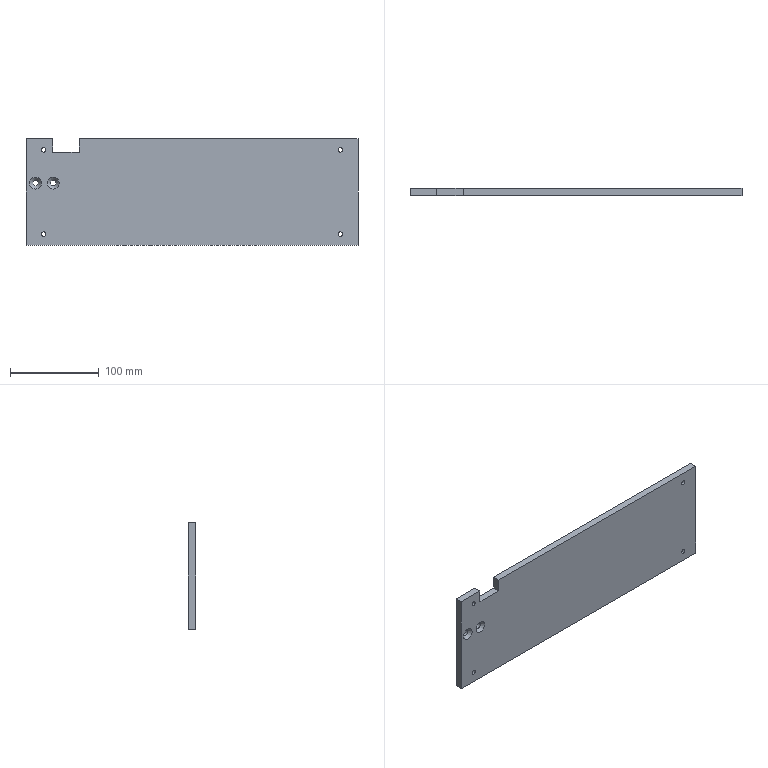Part | NX | features 5003_217_Plate 2 | 1 solid | 18 faces | box 374.6 x 8 x 120 mm | volume 354507 mm3 | plane 10 | cylinder 6 | cone 2 | commonest cylinder face diameters 5 x4 6.6 x2
STEP:
#1=CARTESIAN_POINT('',(-158.775,-14.1,-42.));
#2=VERTEX_POINT('',#1);
#3=CARTESIAN_POINT('',(-128.775,-14.1,-42.));
#4=VERTEX_POINT('',#3);
#5=CARTESIAN_POINT('',(-158.775,-14.1,-42.));
#6=DIRECTION('',(1.,0.,0.));
#7=VECTOR('',#6,1000.);
#8=LINE('',#5,#7);
#9=EDGE_CURVE('',#2,#4,#8,.T.);
#10=ORIENTED_EDGE('',*,*,#9,.T.);
#11=CARTESIAN_POINT('',(-128.775,-6.1,-42.));
#12=VERTEX_POINT('',#11);
#13=CARTESIAN_POINT('',(-128.775,-6.1,-42.));
#14=DIRECTION('',(0.,-1.,0.));
#15=VECTOR('',#14,1000.);
#16=LINE('',#13,#15);
#17=EDGE_CURVE('',#12,#4,#16,.T.);
#18=ORIENTED_EDGE('',*,*,#17,.F.);
#19=CARTESIAN_POINT('',(-158.775,-6.1,-42.));
#20=VERTEX_POINT('',#19);
#21=CARTESIAN_POINT('',(-158.775,-6.1,-42.));
#22=DIRECTION('',(1.,0.,0.));
#23=VECTOR('',#22,1000.);
#24=LINE('',#21,#23);
#25=EDGE_CURVE('',#20,#12,#24,.T.);
#26=ORIENTED_EDGE('',*,*,#25,.F.);
#27=CARTESIAN_POINT('',(-158.775,-6.1,-42.));
#28=DIRECTION('',(0.,-1.,0.));
#29=VECTOR('',#28,1000.);
#30=LINE('',#27,#29);
#31=EDGE_CURVE('',#20,#2,#30,.T.);
#32=ORIENTED_EDGE('',*,*,#31,.T.);
#33=EDGE_LOOP('',(#10,#18,#26,#32));
#34=FACE_BOUND('',#33,.T.);
#35=CARTESIAN_POINT('',(-158.775,-6.1,-42.));
#36=DIRECTION('',(0.,0.,-1.));
#37=DIRECTION('',(-1.,0.,0.));
#38=AXIS2_PLACEMENT_3D('',#35,#36,#37);
#39=PLANE('',#38);
#40=ADVANCED_FACE('',(#34),#39,.F.);
#41=CARTESIAN_POINT('',(-128.775,-14.1,-27.));
#42=VERTEX_POINT('',#41);
#43=CARTESIAN_POINT('',(-128.775,-14.1,-42.));
#44=DIRECTION('',(0.,0.,1.));
#45=VECTOR('',#44,1000.);
#46=LINE('',#43,#45);
#47=EDGE_CURVE('',#4,#42,#46,.T.);
#48=ORIENTED_EDGE('',*,*,#47,.T.);
#49=CARTESIAN_POINT('',(-128.775,-6.1,-27.));
#50=VERTEX_POINT('',#49);
#51=CARTESIAN_POINT('',(-128.775,-6.1,-27.));
#52=DIRECTION('',(0.,-1.,0.));
#53=VECTOR('',#52,1000.);
#54=LINE('',#51,#53);
#55=EDGE_CURVE('',#50,#42,#54,.T.);
#56=ORIENTED_EDGE('',*,*,#55,.F.);
#57=CARTESIAN_POINT('',(-128.775,-6.1,-42.));
#58=DIRECTION('',(0.,0.,1.));
#59=VECTOR('',#58,1000.);
#60=LINE('',#57,#59);
#61=EDGE_CURVE('',#12,#50,#60,.T.);
#62=ORIENTED_EDGE('',*,*,#61,.F.);
#63=ORIENTED_EDGE('',*,*,#17,.T.);
#64=EDGE_LOOP('',(#48,#56,#62,#63));
#65=FACE_BOUND('',#64,.T.);
#66=CARTESIAN_POINT('',(-128.775,-6.1,-42.));
#67=DIRECTION('',(1.,0.,0.));
#68=DIRECTION('',(0.,0.,-1.));
#69=AXIS2_PLACEMENT_3D('',#66,#67,#68);
#70=PLANE('',#69);
#71=ADVANCED_FACE('',(#65),#70,.F.);
#72=CARTESIAN_POINT('',(185.825,-14.1,-27.));
#73=VERTEX_POINT('',#72);
#74=CARTESIAN_POINT('',(-128.775,-14.1,-27.));
#75=DIRECTION('',(1.,0.,0.));
#76=VECTOR('',#75,1000.);
#77=LINE('',#74,#76);
#78=EDGE_CURVE('',#42,#73,#77,.T.);
#79=ORIENTED_EDGE('',*,*,#78,.T.);
#80=CARTESIAN_POINT('',(185.825,-6.1,-27.));
#81=VERTEX_POINT('',#80);
#82=CARTESIAN_POINT('',(185.825,-6.1,-27.));
#83=DIRECTION('',(0.,-1.,0.));
#84=VECTOR('',#83,1000.);
#85=LINE('',#82,#84);
#86=EDGE_CURVE('',#81,#73,#85,.T.);
#87=ORIENTED_EDGE('',*,*,#86,.F.);
#88=CARTESIAN_POINT('',(-128.775,-6.1,-27.));
#89=DIRECTION('',(1.,0.,0.));
#90=VECTOR('',#89,1000.);
#91=LINE('',#88,#90);
#92=EDGE_CURVE('',#50,#81,#91,.T.);
#93=ORIENTED_EDGE('',*,*,#92,.F.);
#94=ORIENTED_EDGE('',*,*,#55,.T.);
#95=EDGE_LOOP('',(#79,#87,#93,#94));
#96=FACE_BOUND('',#95,.T.);
#97=CARTESIAN_POINT('',(-128.775,-6.1,-27.));
#98=DIRECTION('',(0.,0.,-1.));
#99=DIRECTION('',(0.,-1.,0.));
#100=AXIS2_PLACEMENT_3D('',#97,#98,#99);
#101=PLANE('',#100);
#102=ADVANCED_FACE('',(#96),#101,.F.);
#103=CARTESIAN_POINT('',(185.825,-14.1,-147.));
#104=VERTEX_POINT('',#103);
#105=CARTESIAN_POINT('',(185.825,-14.1,-27.));
#106=DIRECTION('',(0.,0.,-1.));
#107=VECTOR('',#106,1000.);
#108=LINE('',#105,#107);
#109=EDGE_CURVE('',#73,#104,#108,.T.);
#110=ORIENTED_EDGE('',*,*,#109,.T.);
#111=CARTESIAN_POINT('',(185.825,-6.1,-147.));
#112=VERTEX_POINT('',#111);
#113=CARTESIAN_POINT('',(185.825,-6.1,-147.));
#114=DIRECTION('',(0.,-1.,0.));
#115=VECTOR('',#114,1000.);
#116=LINE('',#113,#115);
#117=EDGE_CURVE('',#112,#104,#116,.T.);
#118=ORIENTED_EDGE('',*,*,#117,.F.);
#119=CARTESIAN_POINT('',(185.825,-6.1,-27.));
#120=DIRECTION('',(0.,0.,-1.));
#121=VECTOR('',#120,1000.);
#122=LINE('',#119,#121);
#123=EDGE_CURVE('',#81,#112,#122,.T.);
#124=ORIENTED_EDGE('',*,*,#123,.F.);
#125=ORIENTED_EDGE('',*,*,#86,.T.);
#126=EDGE_LOOP('',(#110,#118,#124,#125));
#127=FACE_BOUND('',#126,.T.);
#128=CARTESIAN_POINT('',(185.825,-6.1,-27.));
#129=DIRECTION('',(-1.,0.,0.));
#130=DIRECTION('',(0.,0.,1.));
#131=AXIS2_PLACEMENT_3D('',#128,#129,#130);
#132=PLANE('',#131);
#133=ADVANCED_FACE('',(#127),#132,.F.);
#134=CARTESIAN_POINT('',(-188.775,-14.1,-147.));
#135=VERTEX_POINT('',#134);
#136=CARTESIAN_POINT('',(185.825,-14.1,-147.));
#137=DIRECTION('',(-1.,0.,0.));
#138=VECTOR('',#137,1000.);
#139=LINE('',#136,#138);
#140=EDGE_CURVE('',#104,#135,#139,.T.);
#141=ORIENTED_EDGE('',*,*,#140,.T.);
#142=CARTESIAN_POINT('',(-188.775,-6.1,-147.));
#143=VERTEX_POINT('',#142);
#144=CARTESIAN_POINT('',(-188.775,-6.1,-147.));
#145=DIRECTION('',(0.,-1.,0.));
#146=VECTOR('',#145,1000.);
#147=LINE('',#144,#146);
#148=EDGE_CURVE('',#143,#135,#147,.T.);
#149=ORIENTED_EDGE('',*,*,#148,.F.);
#150=CARTESIAN_POINT('',(185.825,-6.1,-147.));
#151=DIRECTION('',(-1.,0.,0.));
#152=VECTOR('',#151,1000.);
#153=LINE('',#150,#152);
#154=EDGE_CURVE('',#112,#143,#153,.T.);
#155=ORIENTED_EDGE('',*,*,#154,.F.);
#156=ORIENTED_EDGE('',*,*,#117,.T.);
#157=EDGE_LOOP('',(#141,#149,#155,#156));
#158=FACE_BOUND('',#157,.T.);
#159=CARTESIAN_POINT('',(185.825,-6.1,-147.));
#160=DIRECTION('',(0.,0.,1.));
#161=DIRECTION('',(1.,0.,0.));
#162=AXIS2_PLACEMENT_3D('',#159,#160,#161);
#163=PLANE('',#162);
#164=ADVANCED_FACE('',(#158),#163,.F.);
#165=CARTESIAN_POINT('',(-188.775,-14.1,-27.));
#166=VERTEX_POINT('',#165);
#167=CARTESIAN_POINT('',(-188.775,-14.1,-147.));
#168=DIRECTION('',(0.,0.,1.));
#169=VECTOR('',#168,1000.);
#170=LINE('',#167,#169);
#171=EDGE_CURVE('',#135,#166,#170,.T.);
#172=ORIENTED_EDGE('',*,*,#171,.T.);
#173=CARTESIAN_POINT('',(-188.775,-6.1,-27.));
#174=VERTEX_POINT('',#173);
#175=CARTESIAN_POINT('',(-188.775,-6.1,-27.));
#176=DIRECTION('',(0.,-1.,0.));
#177=VECTOR('',#176,1000.);
#178=LINE('',#175,#177);
#179=EDGE_CURVE('',#174,#166,#178,.T.);
#180=ORIENTED_EDGE('',*,*,#179,.F.);
#181=CARTESIAN_POINT('',(-188.775,-6.1,-147.));
#182=DIRECTION('',(0.,0.,1.));
#183=VECTOR('',#182,1000.);
#184=LINE('',#181,#183);
#185=EDGE_CURVE('',#143,#174,#184,.T.);
#186=ORIENTED_EDGE('',*,*,#185,.F.);
#187=ORIENTED_EDGE('',*,*,#148,.T.);
#188=EDGE_LOOP('',(#172,#180,#186,#187));
#189=FACE_BOUND('',#188,.T.);
#190=CARTESIAN_POINT('',(-188.775,-6.1,-147.));
#191=DIRECTION('',(1.,0.,0.));
#192=DIRECTION('',(0.,0.,-1.));
#193=AXIS2_PLACEMENT_3D('',#190,#191,#192);
#194=PLANE('',#193);
#195=ADVANCED_FACE('',(#189),#194,.F.);
#196=CARTESIAN_POINT('',(-158.775,-14.1,-27.));
#197=VERTEX_POINT('',#196);
#198=CARTESIAN_POINT('',(-188.775,-14.1,-27.));
#199=DIRECTION('',(1.,0.,0.));
#200=VECTOR('',#199,1000.);
#201=LINE('',#198,#200);
#202=EDGE_CURVE('',#166,#197,#201,.T.);
#203=ORIENTED_EDGE('',*,*,#202,.T.);
#204=CARTESIAN_POINT('',(-158.775,-6.1,-27.));
#205=VERTEX_POINT('',#204);
#206=CARTESIAN_POINT('',(-158.775,-6.1,-27.));
#207=DIRECTION('',(0.,-1.,0.));
#208=VECTOR('',#207,1000.);
#209=LINE('',#206,#208);
#210=EDGE_CURVE('',#205,#197,#209,.T.);
#211=ORIENTED_EDGE('',*,*,#210,.F.);
#212=CARTESIAN_POINT('',(-188.775,-6.1,-27.));
#213=DIRECTION('',(1.,0.,0.));
#214=VECTOR('',#213,1000.);
#215=LINE('',#212,#214);
#216=EDGE_CURVE('',#174,#205,#215,.T.);
#217=ORIENTED_EDGE('',*,*,#216,.F.);
#218=ORIENTED_EDGE('',*,*,#179,.T.);
#219=EDGE_LOOP('',(#203,#211,#217,#218));
#220=FACE_BOUND('',#219,.T.);
#221=CARTESIAN_POINT('',(-188.775,-6.1,-27.));
#222=DIRECTION('',(0.,0.,-1.));
#223=DIRECTION('',(-1.,0.,0.));
#224=AXIS2_PLACEMENT_3D('',#221,#222,#223);
#225=PLANE('',#224);
#226=ADVANCED_FACE('',(#220),#225,.F.);
#227=CARTESIAN_POINT('',(-158.775,-14.1,-27.));
#228=DIRECTION('',(0.,0.,-1.));
#229=VECTOR('',#228,1000.);
#230=LINE('',#227,#229);
#231=EDGE_CURVE('',#197,#2,#230,.T.);
#232=ORIENTED_EDGE('',*,*,#231,.T.);
#233=ORIENTED_EDGE('',*,*,#31,.F.);
#234=CARTESIAN_POINT('',(-158.775,-6.1,-27.));
#235=DIRECTION('',(0.,0.,-1.));
#236=VECTOR('',#235,1000.);
#237=LINE('',#234,#236);
#238=EDGE_CURVE('',#205,#20,#237,.T.);
#239=ORIENTED_EDGE('',*,*,#238,.F.);
#240=ORIENTED_EDGE('',*,*,#210,.T.);
#241=EDGE_LOOP('',(#232,#233,#239,#240));
#242=FACE_BOUND('',#241,.T.);
#243=CARTESIAN_POINT('',(-158.775,-6.1,-27.));
#244=DIRECTION('',(-1.,0.,0.));
#245=DIRECTION('',(0.,0.,1.));
#246=AXIS2_PLACEMENT_3D('',#243,#244,#245);
#247=PLANE('',#246);
#248=ADVANCED_FACE('',(#242),#247,.F.);
#249=CARTESIAN_POINT('',(-168.775,-6.1,-132.));
#250=VERTEX_POINT('',#249);
#251=CARTESIAN_POINT('',(-168.775,-6.1,-134.5));
#252=DIRECTION('',(0.,-1.,0.));
#253=DIRECTION('',(0.,0.,1.));
#254=AXIS2_PLACEMENT_3D('',#251,#252,#253);
#255=CIRCLE('',#254,2.5);
#256=EDGE_CURVE('',#250,#250,#255,.T.);
#257=ORIENTED_EDGE('',*,*,#256,.T.);
#258=EDGE_LOOP('',(#257));
#259=FACE_BOUND('',#258,.T.);
#260=CARTESIAN_POINT('',(-168.775,-6.1,-37.));
#261=VERTEX_POINT('',#260);
#262=CARTESIAN_POINT('',(-168.775,-6.1,-39.5));
#263=DIRECTION('',(0.,-1.,0.));
#264=DIRECTION('',(0.,0.,1.));
#265=AXIS2_PLACEMENT_3D('',#262,#263,#264);
#266=CIRCLE('',#265,2.5);
#267=EDGE_CURVE('',#261,#261,#266,.T.);
#268=ORIENTED_EDGE('',*,*,#267,.T.);
#269=EDGE_LOOP('',(#268));
#270=FACE_BOUND('',#269,.T.);
#271=CARTESIAN_POINT('',(165.825,-6.1,-37.));
#272=VERTEX_POINT('',#271);
#273=CARTESIAN_POINT('',(165.825,-6.1,-39.5));
#274=DIRECTION('',(0.,-1.,0.));
#275=DIRECTION('',(0.,0.,1.));
#276=AXIS2_PLACEMENT_3D('',#273,#274,#275);
#277=CIRCLE('',#276,2.5);
#278=EDGE_CURVE('',#272,#272,#277,.T.);
#279=ORIENTED_EDGE('',*,*,#278,.T.);
#280=EDGE_LOOP('',(#279));
#281=FACE_BOUND('',#280,.T.);
#282=CARTESIAN_POINT('',(165.825,-6.1,-132.));
#283=VERTEX_POINT('',#282);
#284=CARTESIAN_POINT('',(165.825,-6.1,-134.5));
#285=DIRECTION('',(0.,-1.,0.));
#286=DIRECTION('',(0.,0.,1.));
#287=AXIS2_PLACEMENT_3D('',#284,#285,#286);
#288=CIRCLE('',#287,2.5);
#289=EDGE_CURVE('',#283,#283,#288,.T.);
#290=ORIENTED_EDGE('',*,*,#289,.T.);
#291=EDGE_LOOP('',(#290));
#292=FACE_BOUND('',#291,.T.);
#293=CARTESIAN_POINT('',(-178.115,-6.1,-73.7));
#294=VERTEX_POINT('',#293);
#295=CARTESIAN_POINT('',(-178.115,-6.1,-77.));
#296=DIRECTION('',(0.,-1.,0.));
#297=DIRECTION('',(0.,0.,1.));
#298=AXIS2_PLACEMENT_3D('',#295,#296,#297);
#299=CIRCLE('',#298,3.3);
#300=EDGE_CURVE('',#294,#294,#299,.T.);
#301=ORIENTED_EDGE('',*,*,#300,.T.);
#302=EDGE_LOOP('',(#301));
#303=FACE_BOUND('',#302,.T.);
#304=CARTESIAN_POINT('',(-158.115,-6.1,-73.7));
#305=VERTEX_POINT('',#304);
#306=CARTESIAN_POINT('',(-158.115,-6.1,-77.));
#307=DIRECTION('',(0.,-1.,0.));
#308=DIRECTION('',(0.,0.,1.));
#309=AXIS2_PLACEMENT_3D('',#306,#307,#308);
#310=CIRCLE('',#309,3.3);
#311=EDGE_CURVE('',#305,#305,#310,.T.);
#312=ORIENTED_EDGE('',*,*,#311,.T.);
#313=EDGE_LOOP('',(#312));
#314=FACE_BOUND('',#313,.T.);
#315=ORIENTED_EDGE('',*,*,#25,.T.);
#316=ORIENTED_EDGE('',*,*,#61,.T.);
#317=ORIENTED_EDGE('',*,*,#92,.T.);
#318=ORIENTED_EDGE('',*,*,#123,.T.);
#319=ORIENTED_EDGE('',*,*,#154,.T.);
#320=ORIENTED_EDGE('',*,*,#185,.T.);
#321=ORIENTED_EDGE('',*,*,#216,.T.);
#322=ORIENTED_EDGE('',*,*,#238,.T.);
#323=EDGE_LOOP('',(#315,#316,#317,#318,#319,#320,#321,#322));
#324=FACE_BOUND('',#323,.T.);
#325=CARTESIAN_POINT('',(28.525,-6.1,-27.));
#326=DIRECTION('',(0.,-1.,0.));
#327=DIRECTION('',(0.,0.,1.));
#328=AXIS2_PLACEMENT_3D('',#325,#326,#327);
#329=PLANE('',#328);
#330=ADVANCED_FACE('',(#259,#270,#281,#292,#303,#314,#324),#329,.F.);
#331=CARTESIAN_POINT('',(-168.775,-14.1,-132.));
#332=VERTEX_POINT('',#331);
#333=CARTESIAN_POINT('',(-168.775,-14.1,-134.5));
#334=DIRECTION('',(0.,-1.,0.));
#335=DIRECTION('',(0.,0.,1.));
#336=AXIS2_PLACEMENT_3D('',#333,#334,#335);
#337=CIRCLE('',#336,2.5);
#338=EDGE_CURVE('',#332,#332,#337,.T.);
#339=ORIENTED_EDGE('',*,*,#338,.F.);
#340=EDGE_LOOP('',(#339));
#341=FACE_BOUND('',#340,.T.);
#342=CARTESIAN_POINT('',(-168.775,-14.1,-37.));
#343=VERTEX_POINT('',#342);
#344=CARTESIAN_POINT('',(-168.775,-14.1,-39.5));
#345=DIRECTION('',(0.,-1.,0.));
#346=DIRECTION('',(0.,0.,1.));
#347=AXIS2_PLACEMENT_3D('',#344,#345,#346);
#348=CIRCLE('',#347,2.5);
#349=EDGE_CURVE('',#343,#343,#348,.T.);
#350=ORIENTED_EDGE('',*,*,#349,.F.);
#351=EDGE_LOOP('',(#350));
#352=FACE_BOUND('',#351,.T.);
#353=CARTESIAN_POINT('',(165.825,-14.1,-37.));
#354=VERTEX_POINT('',#353);
#355=CARTESIAN_POINT('',(165.825,-14.1,-39.5));
#356=DIRECTION('',(0.,-1.,0.));
#357=DIRECTION('',(0.,0.,1.));
#358=AXIS2_PLACEMENT_3D('',#355,#356,#357);
#359=CIRCLE('',#358,2.5);
#360=EDGE_CURVE('',#354,#354,#359,.T.);
#361=ORIENTED_EDGE('',*,*,#360,.F.);
#362=EDGE_LOOP('',(#361));
#363=FACE_BOUND('',#362,.T.);
#364=CARTESIAN_POINT('',(165.825,-14.1,-132.));
#365=VERTEX_POINT('',#364);
#366=CARTESIAN_POINT('',(165.825,-14.1,-134.5));
#367=DIRECTION('',(0.,-1.,0.));
#368=DIRECTION('',(0.,0.,1.));
#369=AXIS2_PLACEMENT_3D('',#366,#367,#368);
#370=CIRCLE('',#369,2.5);
#371=EDGE_CURVE('',#365,#365,#370,.T.);
#372=ORIENTED_EDGE('',*,*,#371,.F.);
#373=EDGE_LOOP('',(#372));
#374=FACE_BOUND('',#373,.T.);
#375=CARTESIAN_POINT('',(-178.115,-14.1,-70.25));
#376=VERTEX_POINT('',#375);
#377=CARTESIAN_POINT('',(-178.115,-14.1,-77.));
#378=DIRECTION('',(0.,-1.,0.));
#379=DIRECTION('',(0.,0.,1.));
#380=AXIS2_PLACEMENT_3D('',#377,#378,#379);
#381=CIRCLE('',#380,6.75);
#382=EDGE_CURVE('',#376,#376,#381,.T.);
#383=ORIENTED_EDGE('',*,*,#382,.F.);
#384=EDGE_LOOP('',(#383));
#385=FACE_BOUND('',#384,.T.);
#386=CARTESIAN_POINT('',(-158.115,-14.1,-70.25));
#387=VERTEX_POINT('',#386);
#388=CARTESIAN_POINT('',(-158.115,-14.1,-77.));
#389=DIRECTION('',(0.,-1.,0.));
#390=DIRECTION('',(0.,0.,1.));
#391=AXIS2_PLACEMENT_3D('',#388,#389,#390);
#392=CIRCLE('',#391,6.75);
#393=EDGE_CURVE('',#387,#387,#392,.T.);
#394=ORIENTED_EDGE('',*,*,#393,.F.);
#395=EDGE_LOOP('',(#394));
#396=FACE_BOUND('',#395,.T.);
#397=ORIENTED_EDGE('',*,*,#9,.F.);
#398=ORIENTED_EDGE('',*,*,#231,.F.);
#399=ORIENTED_EDGE('',*,*,#202,.F.);
#400=ORIENTED_EDGE('',*,*,#171,.F.);
#401=ORIENTED_EDGE('',*,*,#140,.F.);
#402=ORIENTED_EDGE('',*,*,#109,.F.);
#403=ORIENTED_EDGE('',*,*,#78,.F.);
#404=ORIENTED_EDGE('',*,*,#47,.F.);
#405=EDGE_LOOP('',(#397,#398,#399,#400,#401,#402,#403,#404));
#406=FACE_BOUND('',#405,.T.);
#407=CARTESIAN_POINT('',(28.525,-14.1,-27.));
#408=DIRECTION('',(0.,-1.,0.));
#409=DIRECTION('',(0.,0.,1.));
#410=AXIS2_PLACEMENT_3D('',#407,#408,#409);
#411=PLANE('',#410);
#412=ADVANCED_FACE('',(#341,#352,#363,#374,#385,#396,#406),#411,.T.);
#413=ORIENTED_EDGE('',*,*,#311,.F.);
#414=EDGE_LOOP('',(#413));
#415=FACE_BOUND('',#414,.T.);
#416=CARTESIAN_POINT('',(-158.115,-10.65,-73.7));
#417=VERTEX_POINT('',#416);
#418=CARTESIAN_POINT('',(-158.115,-10.65,-77.));
#419=DIRECTION('',(0.,-1.,0.));
#420=DIRECTION('',(0.,0.,1.));
#421=AXIS2_PLACEMENT_3D('',#418,#419,#420);
#422=CIRCLE('',#421,3.3);
#423=EDGE_CURVE('',#417,#417,#422,.T.);
#424=ORIENTED_EDGE('',*,*,#423,.T.);
#425=EDGE_LOOP('',(#424));
#426=FACE_BOUND('',#425,.T.);
#427=CARTESIAN_POINT('',(-158.115,-14.1,-77.));
#428=DIRECTION('',(0.,-1.,0.));
#429=DIRECTION('',(0.,0.,1.));
#430=AXIS2_PLACEMENT_3D('',#427,#428,#429);
#431=CYLINDRICAL_SURFACE('',#430,3.3);
#432=ADVANCED_FACE('',(#415,#426),#431,.F.);
#433=ORIENTED_EDGE('',*,*,#423,.F.);
#434=EDGE_LOOP('',(#433));
#435=FACE_BOUND('',#434,.T.);
#436=ORIENTED_EDGE('',*,*,#393,.T.);
#437=EDGE_LOOP('',(#436));
#438=FACE_BOUND('',#437,.T.);
#439=CARTESIAN_POINT('',(-158.115,-14.1,-77.));
#440=DIRECTION('',(0.,-1.,0.));
#441=DIRECTION('',(0.,0.,1.));
#442=AXIS2_PLACEMENT_3D('',#439,#440,#441);
#443=CONICAL_SURFACE('',#442,6.75,0.7854);
#444=ADVANCED_FACE('',(#435,#438),#443,.F.);
#445=ORIENTED_EDGE('',*,*,#300,.F.);
#446=EDGE_LOOP('',(#445));
#447=FACE_BOUND('',#446,.T.);
#448=CARTESIAN_POINT('',(-178.115,-10.65,-73.7));
#449=VERTEX_POINT('',#448);
#450=CARTESIAN_POINT('',(-178.115,-10.65,-77.));
#451=DIRECTION('',(0.,-1.,0.));
#452=DIRECTION('',(0.,0.,1.));
#453=AXIS2_PLACEMENT_3D('',#450,#451,#452);
#454=CIRCLE('',#453,3.3);
#455=EDGE_CURVE('',#449,#449,#454,.T.);
#456=ORIENTED_EDGE('',*,*,#455,.T.);
#457=EDGE_LOOP('',(#456));
#458=FACE_BOUND('',#457,.T.);
#459=CARTESIAN_POINT('',(-178.115,-14.1,-77.));
#460=DIRECTION('',(0.,-1.,0.));
#461=DIRECTION('',(0.,0.,1.));
#462=AXIS2_PLACEMENT_3D('',#459,#460,#461);
#463=CYLINDRICAL_SURFACE('',#462,3.3);
#464=ADVANCED_FACE('',(#447,#458),#463,.F.);
#465=ORIENTED_EDGE('',*,*,#455,.F.);
#466=EDGE_LOOP('',(#465));
#467=FACE_BOUND('',#466,.T.);
#468=ORIENTED_EDGE('',*,*,#382,.T.);
#469=EDGE_LOOP('',(#468));
#470=FACE_BOUND('',#469,.T.);
#471=CARTESIAN_POINT('',(-178.115,-14.1,-77.));
#472=DIRECTION('',(0.,-1.,0.));
#473=DIRECTION('',(0.,0.,1.));
#474=AXIS2_PLACEMENT_3D('',#471,#472,#473);
#475=CONICAL_SURFACE('',#474,6.75,0.7854);
#476=ADVANCED_FACE('',(#467,#470),#475,.F.);
#477=ORIENTED_EDGE('',*,*,#289,.F.);
#478=EDGE_LOOP('',(#477));
#479=FACE_BOUND('',#478,.T.);
#480=ORIENTED_EDGE('',*,*,#371,.T.);
#481=EDGE_LOOP('',(#480));
#482=FACE_BOUND('',#481,.T.);
#483=CARTESIAN_POINT('',(165.825,-14.1,-134.5));
#484=DIRECTION('',(0.,-1.,0.));
#485=DIRECTION('',(0.,0.,1.));
#486=AXIS2_PLACEMENT_3D('',#483,#484,#485);
#487=CYLINDRICAL_SURFACE('',#486,2.5);
#488=ADVANCED_FACE('',(#479,#482),#487,.F.);
#489=ORIENTED_EDGE('',*,*,#278,.F.);
#490=EDGE_LOOP('',(#489));
#491=FACE_BOUND('',#490,.T.);
#492=ORIENTED_EDGE('',*,*,#360,.T.);
#493=EDGE_LOOP('',(#492));
#494=FACE_BOUND('',#493,.T.);
#495=CARTESIAN_POINT('',(165.825,-14.1,-39.5));
#496=DIRECTION('',(0.,-1.,0.));
#497=DIRECTION('',(0.,0.,1.));
#498=AXIS2_PLACEMENT_3D('',#495,#496,#497);
#499=CYLINDRICAL_SURFACE('',#498,2.5);
#500=ADVANCED_FACE('',(#491,#494),#499,.F.);
#501=ORIENTED_EDGE('',*,*,#267,.F.);
#502=EDGE_LOOP('',(#501));
#503=FACE_BOUND('',#502,.T.);
#504=ORIENTED_EDGE('',*,*,#349,.T.);
#505=EDGE_LOOP('',(#504));
#506=FACE_BOUND('',#505,.T.);
#507=CARTESIAN_POINT('',(-168.775,-14.1,-39.5));
#508=DIRECTION('',(0.,-1.,0.));
#509=DIRECTION('',(0.,0.,1.));
#510=AXIS2_PLACEMENT_3D('',#507,#508,#509);
#511=CYLINDRICAL_SURFACE('',#510,2.5);
#512=ADVANCED_FACE('',(#503,#506),#511,.F.);
#513=ORIENTED_EDGE('',*,*,#256,.F.);
#514=EDGE_LOOP('',(#513));
#515=FACE_BOUND('',#514,.T.);
#516=ORIENTED_EDGE('',*,*,#338,.T.);
#517=EDGE_LOOP('',(#516));
#518=FACE_BOUND('',#517,.T.);
#519=CARTESIAN_POINT('',(-168.775,-14.1,-134.5));
#520=DIRECTION('',(0.,-1.,0.));
#521=DIRECTION('',(0.,0.,1.));
#522=AXIS2_PLACEMENT_3D('',#519,#520,#521);
#523=CYLINDRICAL_SURFACE('',#522,2.5);
#524=ADVANCED_FACE('',(#515,#518),#523,.F.);
#525=CLOSED_SHELL('',(#40,#71,#102,#133,#164,#195,#226,#248,#330,#412,#432,#444,#464,#476,#488,#500,#512,#524));
#526=MANIFOLD_SOLID_BREP('',#525);
#527=(LENGTH_UNIT()NAMED_UNIT(*)SI_UNIT(.MILLI.,.METRE.));
#528=UNCERTAINTY_MEASURE_WITH_UNIT(LENGTH_MEASURE(0.00001),#527,'','');
#529=(NAMED_UNIT(*)PLANE_ANGLE_UNIT()SI_UNIT($,.RADIAN.));
#530=(NAMED_UNIT(*)SI_UNIT($,.STERADIAN.)SOLID_ANGLE_UNIT());
#531=(GEOMETRIC_REPRESENTATION_CONTEXT(3)GLOBAL_UNCERTAINTY_ASSIGNED_CONTEXT((#528))GLOBAL_UNIT_ASSIGNED_CONTEXT((#527,#529,#530))REPRESENTATION_CONTEXT('',''));
#532=ADVANCED_BREP_SHAPE_REPRESENTATION('',(#526),#531);